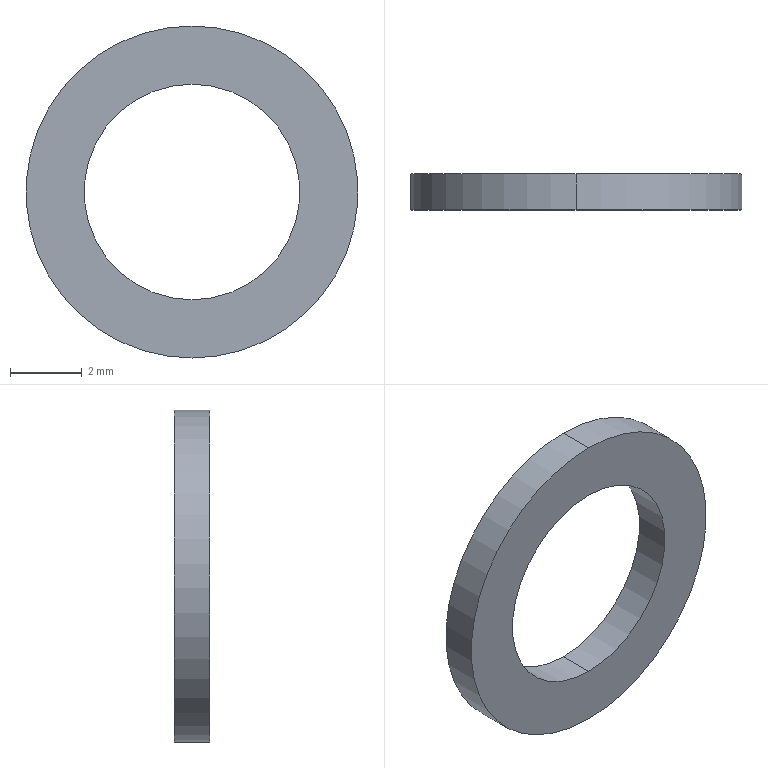Part | NX | features BREP 1 | 1 solid | 6 faces | box 9.238 x 1 x 9.238 mm | volume 38.746 mm3 | cylinder 4 | plane 2 | commonest cylinder face diameters 6 x2 9.238 x2
STEP:
#1=CARTESIAN_POINT('',(0.,1.,-3.));
#2=VERTEX_POINT('',#1);
#3=CARTESIAN_POINT('',(0.,1.,3.));
#4=VERTEX_POINT('',#3);
#5=CARTESIAN_POINT('',(0.,1.,0.));
#6=DIRECTION('',(0.,1.,0.));
#7=DIRECTION('',(0.,0.,1.));
#8=AXIS2_PLACEMENT_3D('',#5,#6,#7);
#9=CIRCLE('',#8,3.);
#10=EDGE_CURVE('',#2,#4,#9,.T.);
#11=ORIENTED_EDGE('',*,*,#10,.T.);
#12=CARTESIAN_POINT('',(0.,0.,3.));
#13=VERTEX_POINT('',#12);
#14=CARTESIAN_POINT('',(0.,1.,3.));
#15=DIRECTION('',(0.,-1.,0.));
#16=VECTOR('',#15,1000.);
#17=LINE('',#14,#16);
#18=EDGE_CURVE('',#13,#4,#17,.F.);
#19=ORIENTED_EDGE('',*,*,#18,.F.);
#20=CARTESIAN_POINT('',(0.,0.,-3.));
#21=VERTEX_POINT('',#20);
#22=CARTESIAN_POINT('',(0.,0.,0.));
#23=DIRECTION('',(0.,1.,0.));
#24=DIRECTION('',(0.,0.,1.));
#25=AXIS2_PLACEMENT_3D('',#22,#23,#24);
#26=CIRCLE('',#25,3.);
#27=EDGE_CURVE('',#21,#13,#26,.T.);
#28=ORIENTED_EDGE('',*,*,#27,.F.);
#29=CARTESIAN_POINT('',(0.,1.,-3.));
#30=DIRECTION('',(0.,-1.,0.));
#31=VECTOR('',#30,1000.);
#32=LINE('',#29,#31);
#33=EDGE_CURVE('',#21,#2,#32,.F.);
#34=ORIENTED_EDGE('',*,*,#33,.T.);
#35=EDGE_LOOP('',(#11,#19,#28,#34));
#36=FACE_BOUND('',#35,.T.);
#37=CARTESIAN_POINT('',(0.,1.,0.));
#38=DIRECTION('',(0.,-1.,0.));
#39=DIRECTION('',(0.,0.,1.));
#40=AXIS2_PLACEMENT_3D('',#37,#38,#39);
#41=CYLINDRICAL_SURFACE('',#40,3.);
#42=ADVANCED_FACE('',(#36),#41,.F.);
#43=CARTESIAN_POINT('',(0.,1.,4.619));
#44=VERTEX_POINT('',#43);
#45=CARTESIAN_POINT('',(0.,1.,-4.619));
#46=VERTEX_POINT('',#45);
#47=CARTESIAN_POINT('',(0.,1.,0.));
#48=DIRECTION('',(0.,1.,0.));
#49=DIRECTION('',(0.,0.,1.));
#50=AXIS2_PLACEMENT_3D('',#47,#48,#49);
#51=CIRCLE('',#50,4.619);
#52=EDGE_CURVE('',#44,#46,#51,.T.);
#53=ORIENTED_EDGE('',*,*,#52,.F.);
#54=CARTESIAN_POINT('',(0.,0.,4.619));
#55=VERTEX_POINT('',#54);
#56=CARTESIAN_POINT('',(0.,1.,4.619));
#57=DIRECTION('',(0.,-1.,0.));
#58=VECTOR('',#57,1000.);
#59=LINE('',#56,#58);
#60=EDGE_CURVE('',#55,#44,#59,.F.);
#61=ORIENTED_EDGE('',*,*,#60,.F.);
#62=CARTESIAN_POINT('',(0.,0.,-4.619));
#63=VERTEX_POINT('',#62);
#64=CARTESIAN_POINT('',(0.,0.,0.));
#65=DIRECTION('',(0.,1.,0.));
#66=DIRECTION('',(0.,0.,1.));
#67=AXIS2_PLACEMENT_3D('',#64,#65,#66);
#68=CIRCLE('',#67,4.619);
#69=EDGE_CURVE('',#55,#63,#68,.T.);
#70=ORIENTED_EDGE('',*,*,#69,.T.);
#71=CARTESIAN_POINT('',(0.,1.,-4.619));
#72=DIRECTION('',(0.,-1.,0.));
#73=VECTOR('',#72,1000.);
#74=LINE('',#71,#73);
#75=EDGE_CURVE('',#63,#46,#74,.F.);
#76=ORIENTED_EDGE('',*,*,#75,.T.);
#77=EDGE_LOOP('',(#53,#61,#70,#76));
#78=FACE_BOUND('',#77,.T.);
#79=CARTESIAN_POINT('',(0.,1.,0.));
#80=DIRECTION('',(0.,-1.,0.));
#81=DIRECTION('',(0.,0.,1.));
#82=AXIS2_PLACEMENT_3D('',#79,#80,#81);
#83=CYLINDRICAL_SURFACE('',#82,4.619);
#84=ADVANCED_FACE('',(#78),#83,.T.);
#85=CARTESIAN_POINT('',(0.,1.,0.));
#86=DIRECTION('',(0.,1.,0.));
#87=DIRECTION('',(0.,0.,1.));
#88=AXIS2_PLACEMENT_3D('',#85,#86,#87);
#89=CIRCLE('',#88,4.619);
#90=EDGE_CURVE('',#46,#44,#89,.T.);
#91=ORIENTED_EDGE('',*,*,#90,.T.);
#92=ORIENTED_EDGE('',*,*,#52,.T.);
#93=EDGE_LOOP('',(#91,#92));
#94=FACE_BOUND('',#93,.T.);
#95=ORIENTED_EDGE('',*,*,#10,.F.);
#96=CARTESIAN_POINT('',(0.,1.,0.));
#97=DIRECTION('',(0.,1.,0.));
#98=DIRECTION('',(0.,0.,1.));
#99=AXIS2_PLACEMENT_3D('',#96,#97,#98);
#100=CIRCLE('',#99,3.);
#101=EDGE_CURVE('',#4,#2,#100,.T.);
#102=ORIENTED_EDGE('',*,*,#101,.F.);
#103=EDGE_LOOP('',(#95,#102));
#104=FACE_BOUND('',#103,.T.);
#105=CARTESIAN_POINT('',(0.,1.,0.));
#106=DIRECTION('',(0.,1.,0.));
#107=DIRECTION('',(0.,0.,1.));
#108=AXIS2_PLACEMENT_3D('',#105,#106,#107);
#109=PLANE('',#108);
#110=ADVANCED_FACE('',(#94,#104),#109,.T.);
#111=CARTESIAN_POINT('',(0.,0.,0.));
#112=DIRECTION('',(0.,1.,0.));
#113=DIRECTION('',(0.,0.,1.));
#114=AXIS2_PLACEMENT_3D('',#111,#112,#113);
#115=CIRCLE('',#114,4.619);
#116=EDGE_CURVE('',#63,#55,#115,.T.);
#117=ORIENTED_EDGE('',*,*,#116,.F.);
#118=ORIENTED_EDGE('',*,*,#69,.F.);
#119=EDGE_LOOP('',(#117,#118));
#120=FACE_BOUND('',#119,.T.);
#121=ORIENTED_EDGE('',*,*,#27,.T.);
#122=CARTESIAN_POINT('',(0.,0.,0.));
#123=DIRECTION('',(0.,1.,0.));
#124=DIRECTION('',(0.,0.,1.));
#125=AXIS2_PLACEMENT_3D('',#122,#123,#124);
#126=CIRCLE('',#125,3.);
#127=EDGE_CURVE('',#13,#21,#126,.T.);
#128=ORIENTED_EDGE('',*,*,#127,.T.);
#129=EDGE_LOOP('',(#121,#128));
#130=FACE_BOUND('',#129,.T.);
#131=CARTESIAN_POINT('',(0.,0.,0.));
#132=DIRECTION('',(0.,1.,0.));
#133=DIRECTION('',(0.,0.,1.));
#134=AXIS2_PLACEMENT_3D('',#131,#132,#133);
#135=PLANE('',#134);
#136=ADVANCED_FACE('',(#120,#130),#135,.F.);
#137=ORIENTED_EDGE('',*,*,#60,.T.);
#138=ORIENTED_EDGE('',*,*,#90,.F.);
#139=ORIENTED_EDGE('',*,*,#75,.F.);
#140=ORIENTED_EDGE('',*,*,#116,.T.);
#141=EDGE_LOOP('',(#137,#138,#139,#140));
#142=FACE_BOUND('',#141,.T.);
#143=CARTESIAN_POINT('',(0.,1.,0.));
#144=DIRECTION('',(0.,-1.,0.));
#145=DIRECTION('',(0.,0.,1.));
#146=AXIS2_PLACEMENT_3D('',#143,#144,#145);
#147=CYLINDRICAL_SURFACE('',#146,4.619);
#148=ADVANCED_FACE('',(#142),#147,.T.);
#149=ORIENTED_EDGE('',*,*,#18,.T.);
#150=ORIENTED_EDGE('',*,*,#101,.T.);
#151=ORIENTED_EDGE('',*,*,#33,.F.);
#152=ORIENTED_EDGE('',*,*,#127,.F.);
#153=EDGE_LOOP('',(#149,#150,#151,#152));
#154=FACE_BOUND('',#153,.T.);
#155=CARTESIAN_POINT('',(0.,1.,0.));
#156=DIRECTION('',(0.,-1.,0.));
#157=DIRECTION('',(0.,0.,1.));
#158=AXIS2_PLACEMENT_3D('',#155,#156,#157);
#159=CYLINDRICAL_SURFACE('',#158,3.);
#160=ADVANCED_FACE('',(#154),#159,.F.);
#161=CLOSED_SHELL('',(#42,#84,#110,#136,#148,#160));
#162=MANIFOLD_SOLID_BREP('',#161);
#163=(LENGTH_UNIT()NAMED_UNIT(*)SI_UNIT(.MILLI.,.METRE.));
#164=UNCERTAINTY_MEASURE_WITH_UNIT(LENGTH_MEASURE(0.00001),#163,'','');
#165=(NAMED_UNIT(*)PLANE_ANGLE_UNIT()SI_UNIT($,.RADIAN.));
#166=(NAMED_UNIT(*)SI_UNIT($,.STERADIAN.)SOLID_ANGLE_UNIT());
#167=(GEOMETRIC_REPRESENTATION_CONTEXT(3)GLOBAL_UNCERTAINTY_ASSIGNED_CONTEXT((#164))GLOBAL_UNIT_ASSIGNED_CONTEXT((#163,#165,#166))REPRESENTATION_CONTEXT('',''));
#168=ADVANCED_BREP_SHAPE_REPRESENTATION('',(#162),#167);